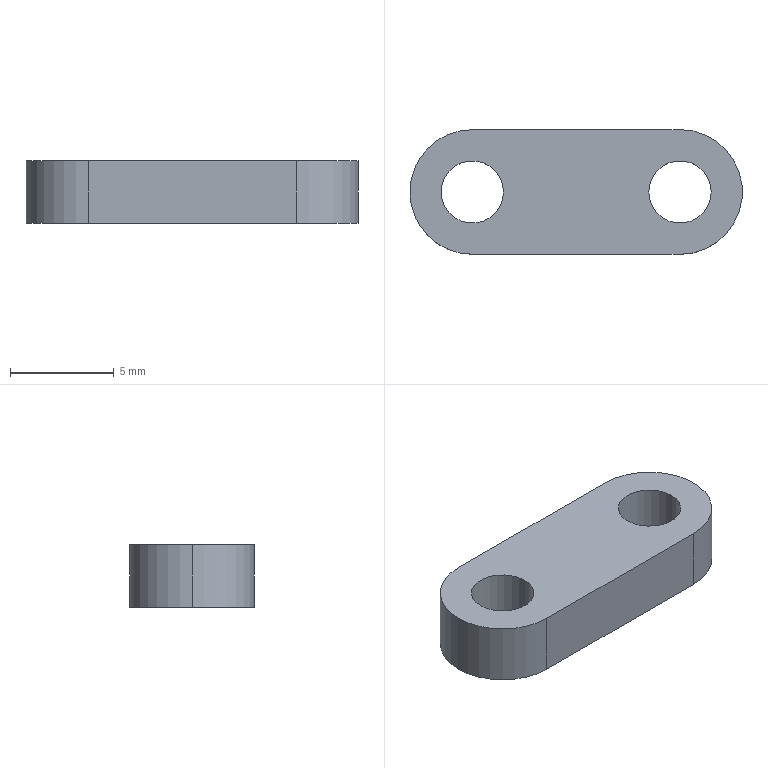Part | SolidWorks | features Extrusion 1 | 1 solid | 11 faces | box 16 x 6 x 3 mm | volume 222.412 mm3 | cylinder 7 | plane 4 | commonest cylinder face diameters 3 x4 6 x3
STEP:
#1=CARTESIAN_POINT('',(8.5,0.,3.));
#2=VERTEX_POINT('',#1);
#3=CARTESIAN_POINT('',(11.5,0.,3.));
#4=VERTEX_POINT('',#3);
#5=CARTESIAN_POINT('',(10.,0.,3.));
#6=DIRECTION('',(0.,0.,1.));
#7=DIRECTION('',(1.,0.,0.));
#8=AXIS2_PLACEMENT_3D('',#5,#6,#7);
#9=CIRCLE('',#8,1.5);
#10=EDGE_CURVE('',#2,#4,#9,.T.);
#11=ORIENTED_EDGE('',*,*,#10,.T.);
#12=CARTESIAN_POINT('',(11.5,0.,0.));
#13=VERTEX_POINT('',#12);
#14=CARTESIAN_POINT('',(11.5,0.,3.));
#15=DIRECTION('',(0.,0.,-1.));
#16=VECTOR('',#15,1000.);
#17=LINE('',#14,#16);
#18=EDGE_CURVE('',#4,#13,#17,.T.);
#19=ORIENTED_EDGE('',*,*,#18,.T.);
#20=CARTESIAN_POINT('',(8.5,0.,0.));
#21=VERTEX_POINT('',#20);
#22=CARTESIAN_POINT('',(10.,0.,0.));
#23=DIRECTION('',(0.,0.,1.));
#24=DIRECTION('',(1.,0.,0.));
#25=AXIS2_PLACEMENT_3D('',#22,#23,#24);
#26=CIRCLE('',#25,1.5);
#27=EDGE_CURVE('',#21,#13,#26,.T.);
#28=ORIENTED_EDGE('',*,*,#27,.F.);
#29=CARTESIAN_POINT('',(8.5,0.,3.));
#30=DIRECTION('',(0.,0.,-1.));
#31=VECTOR('',#30,1000.);
#32=LINE('',#29,#31);
#33=EDGE_CURVE('',#2,#21,#32,.T.);
#34=ORIENTED_EDGE('',*,*,#33,.F.);
#35=EDGE_LOOP('',(#11,#19,#28,#34));
#36=FACE_OUTER_BOUND('',#35,.T.);
#37=CARTESIAN_POINT('',(10.,0.,3.));
#38=DIRECTION('',(0.,0.,-1.));
#39=DIRECTION('',(-1.,0.,0.));
#40=AXIS2_PLACEMENT_3D('',#37,#38,#39);
#41=CYLINDRICAL_SURFACE('',#40,1.5);
#42=ADVANCED_FACE('',(#36),#41,.F.);
#43=CARTESIAN_POINT('',(-1.5,0.,3.));
#44=VERTEX_POINT('',#43);
#45=CARTESIAN_POINT('',(1.5,0.,3.));
#46=VERTEX_POINT('',#45);
#47=CARTESIAN_POINT('',(0.,0.,3.));
#48=DIRECTION('',(0.,0.,1.));
#49=DIRECTION('',(1.,0.,0.));
#50=AXIS2_PLACEMENT_3D('',#47,#48,#49);
#51=CIRCLE('',#50,1.5);
#52=EDGE_CURVE('',#44,#46,#51,.T.);
#53=ORIENTED_EDGE('',*,*,#52,.T.);
#54=CARTESIAN_POINT('',(1.5,0.,0.));
#55=VERTEX_POINT('',#54);
#56=CARTESIAN_POINT('',(1.5,0.,3.));
#57=DIRECTION('',(0.,0.,-1.));
#58=VECTOR('',#57,1000.);
#59=LINE('',#56,#58);
#60=EDGE_CURVE('',#46,#55,#59,.T.);
#61=ORIENTED_EDGE('',*,*,#60,.T.);
#62=CARTESIAN_POINT('',(-1.5,0.,0.));
#63=VERTEX_POINT('',#62);
#64=CARTESIAN_POINT('',(0.,0.,0.));
#65=DIRECTION('',(0.,0.,1.));
#66=DIRECTION('',(1.,0.,0.));
#67=AXIS2_PLACEMENT_3D('',#64,#65,#66);
#68=CIRCLE('',#67,1.5);
#69=EDGE_CURVE('',#63,#55,#68,.T.);
#70=ORIENTED_EDGE('',*,*,#69,.F.);
#71=CARTESIAN_POINT('',(-1.5,0.,3.));
#72=DIRECTION('',(0.,0.,-1.));
#73=VECTOR('',#72,1000.);
#74=LINE('',#71,#73);
#75=EDGE_CURVE('',#44,#63,#74,.T.);
#76=ORIENTED_EDGE('',*,*,#75,.F.);
#77=EDGE_LOOP('',(#53,#61,#70,#76));
#78=FACE_OUTER_BOUND('',#77,.T.);
#79=CARTESIAN_POINT('',(0.,0.,3.));
#80=DIRECTION('',(0.,0.,-1.));
#81=DIRECTION('',(-1.,0.,0.));
#82=AXIS2_PLACEMENT_3D('',#79,#80,#81);
#83=CYLINDRICAL_SURFACE('',#82,1.5);
#84=ADVANCED_FACE('',(#78),#83,.F.);
#85=CARTESIAN_POINT('',(-3.,0.,3.));
#86=VERTEX_POINT('',#85);
#87=CARTESIAN_POINT('',(0.,-3.,3.));
#88=VERTEX_POINT('',#87);
#89=CARTESIAN_POINT('',(0.,0.,3.));
#90=DIRECTION('',(0.,0.,1.));
#91=DIRECTION('',(1.,0.,0.));
#92=AXIS2_PLACEMENT_3D('',#89,#90,#91);
#93=CIRCLE('',#92,3.);
#94=EDGE_CURVE('',#86,#88,#93,.T.);
#95=ORIENTED_EDGE('',*,*,#94,.F.);
#96=CARTESIAN_POINT('',(-3.,0.,0.));
#97=VERTEX_POINT('',#96);
#98=CARTESIAN_POINT('',(-3.,0.,3.));
#99=DIRECTION('',(0.,0.,-1.));
#100=VECTOR('',#99,1000.);
#101=LINE('',#98,#100);
#102=EDGE_CURVE('',#86,#97,#101,.T.);
#103=ORIENTED_EDGE('',*,*,#102,.T.);
#104=CARTESIAN_POINT('',(0.,-3.,0.));
#105=VERTEX_POINT('',#104);
#106=CARTESIAN_POINT('',(0.,0.,0.));
#107=DIRECTION('',(0.,0.,1.));
#108=DIRECTION('',(1.,0.,0.));
#109=AXIS2_PLACEMENT_3D('',#106,#107,#108);
#110=CIRCLE('',#109,3.);
#111=EDGE_CURVE('',#97,#105,#110,.T.);
#112=ORIENTED_EDGE('',*,*,#111,.T.);
#113=CARTESIAN_POINT('',(0.,-3.,3.));
#114=DIRECTION('',(0.,0.,-1.));
#115=VECTOR('',#114,1000.);
#116=LINE('',#113,#115);
#117=EDGE_CURVE('',#88,#105,#116,.T.);
#118=ORIENTED_EDGE('',*,*,#117,.F.);
#119=EDGE_LOOP('',(#95,#103,#112,#118));
#120=FACE_OUTER_BOUND('',#119,.T.);
#121=CARTESIAN_POINT('',(0.,0.,3.));
#122=DIRECTION('',(0.,0.,-1.));
#123=DIRECTION('',(-1.,0.,0.));
#124=AXIS2_PLACEMENT_3D('',#121,#122,#123);
#125=CYLINDRICAL_SURFACE('',#124,3.);
#126=ADVANCED_FACE('',(#120),#125,.T.);
#127=ORIENTED_EDGE('',*,*,#52,.F.);
#128=CARTESIAN_POINT('',(0.,0.,3.));
#129=DIRECTION('',(0.,0.,1.));
#130=DIRECTION('',(1.,0.,0.));
#131=AXIS2_PLACEMENT_3D('',#128,#129,#130);
#132=CIRCLE('',#131,1.5);
#133=EDGE_CURVE('',#46,#44,#132,.T.);
#134=ORIENTED_EDGE('',*,*,#133,.F.);
#135=EDGE_LOOP('',(#127,#134));
#136=FACE_BOUND('',#135,.T.);
#137=CARTESIAN_POINT('',(0.,3.,3.));
#138=VERTEX_POINT('',#137);
#139=CARTESIAN_POINT('',(0.,0.,3.));
#140=DIRECTION('',(0.,0.,1.));
#141=DIRECTION('',(1.,0.,0.));
#142=AXIS2_PLACEMENT_3D('',#139,#140,#141);
#143=CIRCLE('',#142,3.);
#144=EDGE_CURVE('',#138,#86,#143,.T.);
#145=ORIENTED_EDGE('',*,*,#144,.T.);
#146=ORIENTED_EDGE('',*,*,#94,.T.);
#147=CARTESIAN_POINT('',(10.,-3.,3.));
#148=VERTEX_POINT('',#147);
#149=CARTESIAN_POINT('',(0.,-3.,3.));
#150=DIRECTION('',(1.,0.,0.));
#151=VECTOR('',#150,1000.);
#152=LINE('',#149,#151);
#153=EDGE_CURVE('',#88,#148,#152,.T.);
#154=ORIENTED_EDGE('',*,*,#153,.T.);
#155=CARTESIAN_POINT('',(10.,3.,3.));
#156=VERTEX_POINT('',#155);
#157=CARTESIAN_POINT('',(10.,0.,3.));
#158=DIRECTION('',(0.,0.,1.));
#159=DIRECTION('',(1.,0.,0.));
#160=AXIS2_PLACEMENT_3D('',#157,#158,#159);
#161=CIRCLE('',#160,3.);
#162=EDGE_CURVE('',#148,#156,#161,.T.);
#163=ORIENTED_EDGE('',*,*,#162,.T.);
#164=CARTESIAN_POINT('',(0.,3.,3.));
#165=DIRECTION('',(-1.,0.,0.));
#166=VECTOR('',#165,1000.);
#167=LINE('',#164,#166);
#168=EDGE_CURVE('',#156,#138,#167,.T.);
#169=ORIENTED_EDGE('',*,*,#168,.T.);
#170=EDGE_LOOP('',(#145,#146,#154,#163,#169));
#171=FACE_OUTER_BOUND('',#170,.T.);
#172=ORIENTED_EDGE('',*,*,#10,.F.);
#173=CARTESIAN_POINT('',(10.,0.,3.));
#174=DIRECTION('',(0.,0.,1.));
#175=DIRECTION('',(1.,0.,0.));
#176=AXIS2_PLACEMENT_3D('',#173,#174,#175);
#177=CIRCLE('',#176,1.5);
#178=EDGE_CURVE('',#4,#2,#177,.T.);
#179=ORIENTED_EDGE('',*,*,#178,.F.);
#180=EDGE_LOOP('',(#172,#179));
#181=FACE_BOUND('',#180,.T.);
#182=CARTESIAN_POINT('',(0.,0.,3.));
#183=DIRECTION('',(0.,0.,1.));
#184=DIRECTION('',(1.,0.,0.));
#185=AXIS2_PLACEMENT_3D('',#182,#183,#184);
#186=PLANE('',#185);
#187=ADVANCED_FACE('',(#136,#171,#181),#186,.T.);
#188=CARTESIAN_POINT('',(0.,3.,0.));
#189=VERTEX_POINT('',#188);
#190=CARTESIAN_POINT('',(0.,0.,0.));
#191=DIRECTION('',(0.,0.,1.));
#192=DIRECTION('',(1.,0.,0.));
#193=AXIS2_PLACEMENT_3D('',#190,#191,#192);
#194=CIRCLE('',#193,3.);
#195=EDGE_CURVE('',#189,#97,#194,.T.);
#196=ORIENTED_EDGE('',*,*,#195,.F.);
#197=CARTESIAN_POINT('',(10.,3.,0.));
#198=VERTEX_POINT('',#197);
#199=CARTESIAN_POINT('',(0.,3.,0.));
#200=DIRECTION('',(-1.,0.,0.));
#201=VECTOR('',#200,1000.);
#202=LINE('',#199,#201);
#203=EDGE_CURVE('',#198,#189,#202,.T.);
#204=ORIENTED_EDGE('',*,*,#203,.F.);
#205=CARTESIAN_POINT('',(10.,-3.,0.));
#206=VERTEX_POINT('',#205);
#207=CARTESIAN_POINT('',(10.,0.,0.));
#208=DIRECTION('',(0.,0.,1.));
#209=DIRECTION('',(1.,0.,0.));
#210=AXIS2_PLACEMENT_3D('',#207,#208,#209);
#211=CIRCLE('',#210,3.);
#212=EDGE_CURVE('',#206,#198,#211,.T.);
#213=ORIENTED_EDGE('',*,*,#212,.F.);
#214=CARTESIAN_POINT('',(0.,-3.,0.));
#215=DIRECTION('',(1.,0.,0.));
#216=VECTOR('',#215,1000.);
#217=LINE('',#214,#216);
#218=EDGE_CURVE('',#105,#206,#217,.T.);
#219=ORIENTED_EDGE('',*,*,#218,.F.);
#220=ORIENTED_EDGE('',*,*,#111,.F.);
#221=EDGE_LOOP('',(#196,#204,#213,#219,#220));
#222=FACE_OUTER_BOUND('',#221,.T.);
#223=ORIENTED_EDGE('',*,*,#69,.T.);
#224=CARTESIAN_POINT('',(0.,0.,0.));
#225=DIRECTION('',(0.,0.,1.));
#226=DIRECTION('',(1.,0.,0.));
#227=AXIS2_PLACEMENT_3D('',#224,#225,#226);
#228=CIRCLE('',#227,1.5);
#229=EDGE_CURVE('',#55,#63,#228,.T.);
#230=ORIENTED_EDGE('',*,*,#229,.T.);
#231=EDGE_LOOP('',(#223,#230));
#232=FACE_BOUND('',#231,.T.);
#233=ORIENTED_EDGE('',*,*,#27,.T.);
#234=CARTESIAN_POINT('',(10.,0.,0.));
#235=DIRECTION('',(0.,0.,1.));
#236=DIRECTION('',(1.,0.,0.));
#237=AXIS2_PLACEMENT_3D('',#234,#235,#236);
#238=CIRCLE('',#237,1.5);
#239=EDGE_CURVE('',#13,#21,#238,.T.);
#240=ORIENTED_EDGE('',*,*,#239,.T.);
#241=EDGE_LOOP('',(#233,#240));
#242=FACE_BOUND('',#241,.T.);
#243=CARTESIAN_POINT('',(0.,0.,0.));
#244=DIRECTION('',(0.,0.,1.));
#245=DIRECTION('',(1.,0.,0.));
#246=AXIS2_PLACEMENT_3D('',#243,#244,#245);
#247=PLANE('',#246);
#248=ADVANCED_FACE('',(#222,#232,#242),#247,.F.);
#249=ORIENTED_EDGE('',*,*,#102,.F.);
#250=ORIENTED_EDGE('',*,*,#144,.F.);
#251=CARTESIAN_POINT('',(0.,3.,3.));
#252=DIRECTION('',(0.,0.,-1.));
#253=VECTOR('',#252,1000.);
#254=LINE('',#251,#253);
#255=EDGE_CURVE('',#138,#189,#254,.T.);
#256=ORIENTED_EDGE('',*,*,#255,.T.);
#257=ORIENTED_EDGE('',*,*,#195,.T.);
#258=EDGE_LOOP('',(#249,#250,#256,#257));
#259=FACE_OUTER_BOUND('',#258,.T.);
#260=CARTESIAN_POINT('',(0.,0.,3.));
#261=DIRECTION('',(0.,0.,-1.));
#262=DIRECTION('',(-1.,0.,0.));
#263=AXIS2_PLACEMENT_3D('',#260,#261,#262);
#264=CYLINDRICAL_SURFACE('',#263,3.);
#265=ADVANCED_FACE('',(#259),#264,.T.);
#266=ORIENTED_EDGE('',*,*,#218,.T.);
#267=CARTESIAN_POINT('',(10.,-3.,3.));
#268=DIRECTION('',(0.,0.,-1.));
#269=VECTOR('',#268,1000.);
#270=LINE('',#267,#269);
#271=EDGE_CURVE('',#148,#206,#270,.T.);
#272=ORIENTED_EDGE('',*,*,#271,.F.);
#273=ORIENTED_EDGE('',*,*,#153,.F.);
#274=ORIENTED_EDGE('',*,*,#117,.T.);
#275=EDGE_LOOP('',(#266,#272,#273,#274));
#276=FACE_OUTER_BOUND('',#275,.T.);
#277=CARTESIAN_POINT('',(0.,-3.,3.));
#278=DIRECTION('',(0.,1.,0.));
#279=DIRECTION('',(0.,0.,1.));
#280=AXIS2_PLACEMENT_3D('',#277,#278,#279);
#281=PLANE('',#280);
#282=ADVANCED_FACE('',(#276),#281,.F.);
#283=ORIENTED_EDGE('',*,*,#212,.T.);
#284=CARTESIAN_POINT('',(10.,3.,3.));
#285=DIRECTION('',(0.,0.,-1.));
#286=VECTOR('',#285,1000.);
#287=LINE('',#284,#286);
#288=EDGE_CURVE('',#156,#198,#287,.T.);
#289=ORIENTED_EDGE('',*,*,#288,.F.);
#290=ORIENTED_EDGE('',*,*,#162,.F.);
#291=ORIENTED_EDGE('',*,*,#271,.T.);
#292=EDGE_LOOP('',(#283,#289,#290,#291));
#293=FACE_OUTER_BOUND('',#292,.T.);
#294=CARTESIAN_POINT('',(10.,0.,3.));
#295=DIRECTION('',(0.,0.,-1.));
#296=DIRECTION('',(-1.,0.,0.));
#297=AXIS2_PLACEMENT_3D('',#294,#295,#296);
#298=CYLINDRICAL_SURFACE('',#297,3.);
#299=ADVANCED_FACE('',(#293),#298,.T.);
#300=ORIENTED_EDGE('',*,*,#203,.T.);
#301=ORIENTED_EDGE('',*,*,#255,.F.);
#302=ORIENTED_EDGE('',*,*,#168,.F.);
#303=ORIENTED_EDGE('',*,*,#288,.T.);
#304=EDGE_LOOP('',(#300,#301,#302,#303));
#305=FACE_OUTER_BOUND('',#304,.T.);
#306=CARTESIAN_POINT('',(0.,3.,3.));
#307=DIRECTION('',(0.,-1.,0.));
#308=DIRECTION('',(0.,0.,-1.));
#309=AXIS2_PLACEMENT_3D('',#306,#307,#308);
#310=PLANE('',#309);
#311=ADVANCED_FACE('',(#305),#310,.F.);
#312=ORIENTED_EDGE('',*,*,#60,.F.);
#313=ORIENTED_EDGE('',*,*,#133,.T.);
#314=ORIENTED_EDGE('',*,*,#75,.T.);
#315=ORIENTED_EDGE('',*,*,#229,.F.);
#316=EDGE_LOOP('',(#312,#313,#314,#315));
#317=FACE_OUTER_BOUND('',#316,.T.);
#318=CARTESIAN_POINT('',(0.,0.,3.));
#319=DIRECTION('',(0.,0.,-1.));
#320=DIRECTION('',(-1.,0.,0.));
#321=AXIS2_PLACEMENT_3D('',#318,#319,#320);
#322=CYLINDRICAL_SURFACE('',#321,1.5);
#323=ADVANCED_FACE('',(#317),#322,.F.);
#324=ORIENTED_EDGE('',*,*,#18,.F.);
#325=ORIENTED_EDGE('',*,*,#178,.T.);
#326=ORIENTED_EDGE('',*,*,#33,.T.);
#327=ORIENTED_EDGE('',*,*,#239,.F.);
#328=EDGE_LOOP('',(#324,#325,#326,#327));
#329=FACE_OUTER_BOUND('',#328,.T.);
#330=CARTESIAN_POINT('',(10.,0.,3.));
#331=DIRECTION('',(0.,0.,-1.));
#332=DIRECTION('',(-1.,0.,0.));
#333=AXIS2_PLACEMENT_3D('',#330,#331,#332);
#334=CYLINDRICAL_SURFACE('',#333,1.5);
#335=ADVANCED_FACE('',(#329),#334,.F.);
#336=CLOSED_SHELL('',(#42,#84,#126,#187,#248,#265,#282,#299,#311,#323,#335));
#337=MANIFOLD_SOLID_BREP('',#336);
#338=CARTESIAN_POINT('',(0.,0.,0.));
#339=DIRECTION('',(0.,0.,1.));
#340=DIRECTION('',(1.,0.,0.));
#341=AXIS2_PLACEMENT_3D('',#338,#339,#340);
#342=(LENGTH_UNIT()NAMED_UNIT(*)SI_UNIT(.MILLI.,.METRE.));
#343=UNCERTAINTY_MEASURE_WITH_UNIT(LENGTH_MEASURE(0.00001),#342,'','');
#344=(NAMED_UNIT(*)PLANE_ANGLE_UNIT()SI_UNIT($,.RADIAN.));
#345=(NAMED_UNIT(*)SI_UNIT($,.STERADIAN.)SOLID_ANGLE_UNIT());
#346=(GEOMETRIC_REPRESENTATION_CONTEXT(3)GLOBAL_UNCERTAINTY_ASSIGNED_CONTEXT((#343))GLOBAL_UNIT_ASSIGNED_CONTEXT((#342,#344,#345))REPRESENTATION_CONTEXT('',''));
#347=ADVANCED_BREP_SHAPE_REPRESENTATION('',(#337,#341),#346);